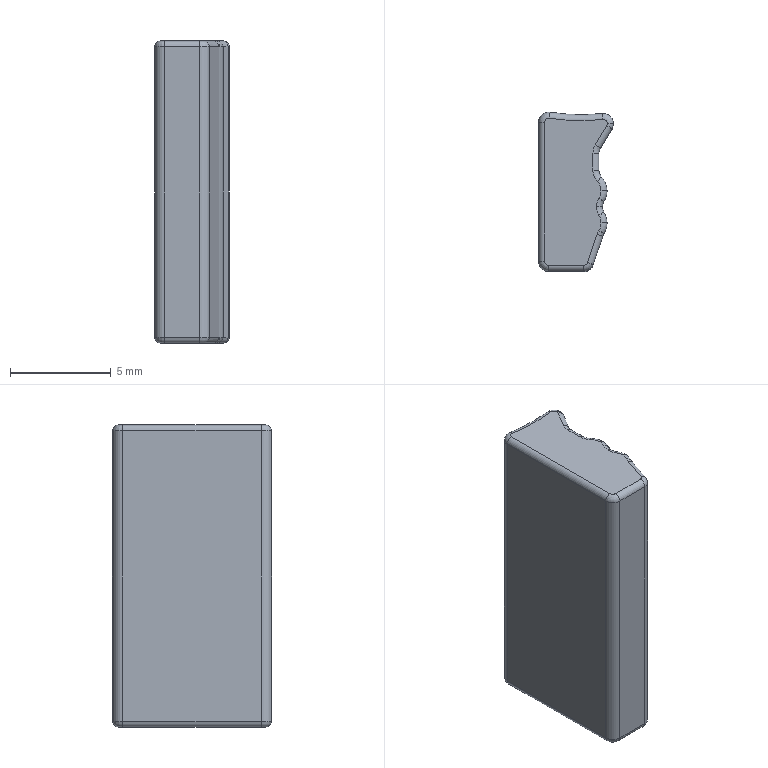Part | STEP file | 101000007616 | 1 solid | 62 faces | box 3.719 x 7.9 x 15 mm | volume 372.862 mm3 | torus 30 | cylinder 25 | plane 7 | commonest cylinder face diameters 0.6 x10 1 x10 2 x4 20 x1